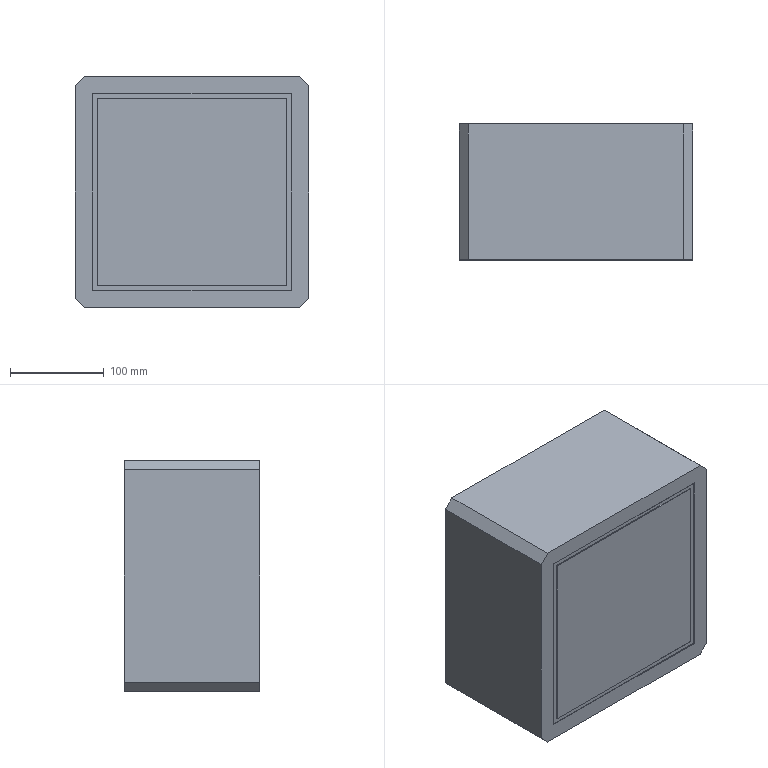Part | SolidWorks | features Chamfer 1, Extrusion 1, ICE 1 | 1 solid | 20 faces | box 250 x 145 x 247 mm | volume 8920630 mm3 | plane 20
STEP:
#1=CARTESIAN_POINT('',(125.,145.,113.5));
#2=VERTEX_POINT('',#1);
#3=CARTESIAN_POINT('',(125.,145.,-113.5));
#4=VERTEX_POINT('',#3);
#5=CARTESIAN_POINT('',(125.,145.,123.5));
#6=DIRECTION('',(0.,0.,-1.));
#7=VECTOR('',#6,1000.);
#8=LINE('',#5,#7);
#9=EDGE_CURVE('',#2,#4,#8,.T.);
#10=ORIENTED_EDGE('',*,*,#9,.F.);
#11=CARTESIAN_POINT('',(125.,0.,113.5));
#12=VERTEX_POINT('',#11);
#13=CARTESIAN_POINT('',(125.,145.,113.5));
#14=DIRECTION('',(0.,-1.,0.));
#15=VECTOR('',#14,1000.);
#16=LINE('',#13,#15);
#17=EDGE_CURVE('',#2,#12,#16,.T.);
#18=ORIENTED_EDGE('',*,*,#17,.T.);
#19=CARTESIAN_POINT('',(125.,0.,-113.5));
#20=VERTEX_POINT('',#19);
#21=CARTESIAN_POINT('',(125.,0.,123.5));
#22=DIRECTION('',(0.,0.,-1.));
#23=VECTOR('',#22,1000.);
#24=LINE('',#21,#23);
#25=EDGE_CURVE('',#12,#20,#24,.T.);
#26=ORIENTED_EDGE('',*,*,#25,.T.);
#27=CARTESIAN_POINT('',(125.,145.,-113.5));
#28=DIRECTION('',(0.,1.,0.));
#29=VECTOR('',#28,1000.);
#30=LINE('',#27,#29);
#31=EDGE_CURVE('',#20,#4,#30,.T.);
#32=ORIENTED_EDGE('',*,*,#31,.T.);
#33=EDGE_LOOP('',(#10,#18,#26,#32));
#34=FACE_OUTER_BOUND('',#33,.T.);
#35=CARTESIAN_POINT('',(125.,145.,123.5));
#36=DIRECTION('',(-1.,0.,0.));
#37=DIRECTION('',(0.,0.,1.));
#38=AXIS2_PLACEMENT_3D('',#35,#36,#37);
#39=PLANE('',#38);
#40=ADVANCED_FACE('',(#34),#39,.F.);
#41=CARTESIAN_POINT('',(115.,145.,-123.5));
#42=VERTEX_POINT('',#41);
#43=CARTESIAN_POINT('',(-115.,145.,-123.5));
#44=VERTEX_POINT('',#43);
#45=CARTESIAN_POINT('',(-125.,145.,-123.5));
#46=DIRECTION('',(-1.,0.,0.));
#47=VECTOR('',#46,1000.);
#48=LINE('',#45,#47);
#49=EDGE_CURVE('',#42,#44,#48,.T.);
#50=ORIENTED_EDGE('',*,*,#49,.F.);
#51=CARTESIAN_POINT('',(115.,0.,-123.5));
#52=VERTEX_POINT('',#51);
#53=CARTESIAN_POINT('',(115.,145.,-123.5));
#54=DIRECTION('',(0.,-1.,0.));
#55=VECTOR('',#54,1000.);
#56=LINE('',#53,#55);
#57=EDGE_CURVE('',#42,#52,#56,.T.);
#58=ORIENTED_EDGE('',*,*,#57,.T.);
#59=CARTESIAN_POINT('',(-115.,0.,-123.5));
#60=VERTEX_POINT('',#59);
#61=CARTESIAN_POINT('',(-125.,0.,-123.5));
#62=DIRECTION('',(-1.,0.,0.));
#63=VECTOR('',#62,1000.);
#64=LINE('',#61,#63);
#65=EDGE_CURVE('',#52,#60,#64,.T.);
#66=ORIENTED_EDGE('',*,*,#65,.T.);
#67=CARTESIAN_POINT('',(-115.,145.,-123.5));
#68=DIRECTION('',(0.,1.,0.));
#69=VECTOR('',#68,1000.);
#70=LINE('',#67,#69);
#71=EDGE_CURVE('',#60,#44,#70,.T.);
#72=ORIENTED_EDGE('',*,*,#71,.T.);
#73=EDGE_LOOP('',(#50,#58,#66,#72));
#74=FACE_OUTER_BOUND('',#73,.T.);
#75=CARTESIAN_POINT('',(-125.,145.,-123.5));
#76=DIRECTION('',(0.,0.,1.));
#77=DIRECTION('',(1.,0.,0.));
#78=AXIS2_PLACEMENT_3D('',#75,#76,#77);
#79=PLANE('',#78);
#80=ADVANCED_FACE('',(#74),#79,.F.);
#81=CARTESIAN_POINT('',(-125.,145.,-113.5));
#82=VERTEX_POINT('',#81);
#83=CARTESIAN_POINT('',(-125.,145.,113.5));
#84=VERTEX_POINT('',#83);
#85=CARTESIAN_POINT('',(-125.,145.,123.5));
#86=DIRECTION('',(0.,0.,1.));
#87=VECTOR('',#86,1000.);
#88=LINE('',#85,#87);
#89=EDGE_CURVE('',#82,#84,#88,.T.);
#90=ORIENTED_EDGE('',*,*,#89,.F.);
#91=CARTESIAN_POINT('',(-125.,0.,-113.5));
#92=VERTEX_POINT('',#91);
#93=CARTESIAN_POINT('',(-125.,145.,-113.5));
#94=DIRECTION('',(0.,-1.,0.));
#95=VECTOR('',#94,1000.);
#96=LINE('',#93,#95);
#97=EDGE_CURVE('',#82,#92,#96,.T.);
#98=ORIENTED_EDGE('',*,*,#97,.T.);
#99=CARTESIAN_POINT('',(-125.,0.,113.5));
#100=VERTEX_POINT('',#99);
#101=CARTESIAN_POINT('',(-125.,0.,123.5));
#102=DIRECTION('',(0.,0.,1.));
#103=VECTOR('',#102,1000.);
#104=LINE('',#101,#103);
#105=EDGE_CURVE('',#92,#100,#104,.T.);
#106=ORIENTED_EDGE('',*,*,#105,.T.);
#107=CARTESIAN_POINT('',(-125.,145.,113.5));
#108=DIRECTION('',(0.,1.,0.));
#109=VECTOR('',#108,1000.);
#110=LINE('',#107,#109);
#111=EDGE_CURVE('',#100,#84,#110,.T.);
#112=ORIENTED_EDGE('',*,*,#111,.T.);
#113=EDGE_LOOP('',(#90,#98,#106,#112));
#114=FACE_OUTER_BOUND('',#113,.T.);
#115=CARTESIAN_POINT('',(-125.,145.,123.5));
#116=DIRECTION('',(1.,0.,0.));
#117=DIRECTION('',(0.,0.,-1.));
#118=AXIS2_PLACEMENT_3D('',#115,#116,#117);
#119=PLANE('',#118);
#120=ADVANCED_FACE('',(#114),#119,.F.);
#121=CARTESIAN_POINT('',(-115.,0.,123.5));
#122=VERTEX_POINT('',#121);
#123=CARTESIAN_POINT('',(115.,0.,123.5));
#124=VERTEX_POINT('',#123);
#125=CARTESIAN_POINT('',(-125.,0.,123.5));
#126=DIRECTION('',(1.,0.,0.));
#127=VECTOR('',#126,1000.);
#128=LINE('',#125,#127);
#129=EDGE_CURVE('',#122,#124,#128,.T.);
#130=ORIENTED_EDGE('',*,*,#129,.T.);
#131=CARTESIAN_POINT('',(115.,145.,123.5));
#132=VERTEX_POINT('',#131);
#133=CARTESIAN_POINT('',(115.,145.,123.5));
#134=DIRECTION('',(0.,1.,0.));
#135=VECTOR('',#134,1000.);
#136=LINE('',#133,#135);
#137=EDGE_CURVE('',#124,#132,#136,.T.);
#138=ORIENTED_EDGE('',*,*,#137,.T.);
#139=CARTESIAN_POINT('',(-115.,145.,123.5));
#140=VERTEX_POINT('',#139);
#141=CARTESIAN_POINT('',(-125.,145.,123.5));
#142=DIRECTION('',(1.,0.,0.));
#143=VECTOR('',#142,1000.);
#144=LINE('',#141,#143);
#145=EDGE_CURVE('',#140,#132,#144,.T.);
#146=ORIENTED_EDGE('',*,*,#145,.F.);
#147=CARTESIAN_POINT('',(-115.,145.,123.5));
#148=DIRECTION('',(0.,-1.,0.));
#149=VECTOR('',#148,1000.);
#150=LINE('',#147,#149);
#151=EDGE_CURVE('',#140,#122,#150,.T.);
#152=ORIENTED_EDGE('',*,*,#151,.T.);
#153=EDGE_LOOP('',(#130,#138,#146,#152));
#154=FACE_OUTER_BOUND('',#153,.T.);
#155=CARTESIAN_POINT('',(-125.,145.,123.5));
#156=DIRECTION('',(0.,0.,-1.));
#157=DIRECTION('',(-1.,0.,0.));
#158=AXIS2_PLACEMENT_3D('',#155,#156,#157);
#159=PLANE('',#158);
#160=ADVANCED_FACE('',(#154),#159,.F.);
#161=ORIENTED_EDGE('',*,*,#145,.T.);
#162=CARTESIAN_POINT('',(125.,145.,113.5));
#163=DIRECTION('',(0.7071,0.,-0.7071));
#164=VECTOR('',#163,1000.);
#165=LINE('',#162,#164);
#166=EDGE_CURVE('',#132,#2,#165,.T.);
#167=ORIENTED_EDGE('',*,*,#166,.T.);
#168=ORIENTED_EDGE('',*,*,#9,.T.);
#169=CARTESIAN_POINT('',(115.,145.,-123.5));
#170=DIRECTION('',(-0.7071,0.,-0.7071));
#171=VECTOR('',#170,1000.);
#172=LINE('',#169,#171);
#173=EDGE_CURVE('',#4,#42,#172,.T.);
#174=ORIENTED_EDGE('',*,*,#173,.T.);
#175=ORIENTED_EDGE('',*,*,#49,.T.);
#176=CARTESIAN_POINT('',(-125.,145.,-113.5));
#177=DIRECTION('',(-0.7071,0.,0.7071));
#178=VECTOR('',#177,1000.);
#179=LINE('',#176,#178);
#180=EDGE_CURVE('',#44,#82,#179,.T.);
#181=ORIENTED_EDGE('',*,*,#180,.T.);
#182=ORIENTED_EDGE('',*,*,#89,.T.);
#183=CARTESIAN_POINT('',(-115.,145.,123.5));
#184=DIRECTION('',(0.7071,0.,0.7071));
#185=VECTOR('',#184,1000.);
#186=LINE('',#183,#185);
#187=EDGE_CURVE('',#84,#140,#186,.T.);
#188=ORIENTED_EDGE('',*,*,#187,.T.);
#189=EDGE_LOOP('',(#161,#167,#168,#174,#175,#181,#182,#188));
#190=FACE_OUTER_BOUND('',#189,.T.);
#191=CARTESIAN_POINT('',(0.,145.,0.));
#192=DIRECTION('',(0.,-1.,0.));
#193=DIRECTION('',(0.,0.,-1.));
#194=AXIS2_PLACEMENT_3D('',#191,#192,#193);
#195=PLANE('',#194);
#196=ADVANCED_FACE('',(#190),#195,.F.);
#197=CARTESIAN_POINT('',(106.,0.,-105.));
#198=VERTEX_POINT('',#197);
#199=CARTESIAN_POINT('',(106.,0.,105.));
#200=VERTEX_POINT('',#199);
#201=CARTESIAN_POINT('',(106.,0.,-105.));
#202=DIRECTION('',(0.,0.,1.));
#203=VECTOR('',#202,1000.);
#204=LINE('',#201,#203);
#205=EDGE_CURVE('',#198,#200,#204,.T.);
#206=ORIENTED_EDGE('',*,*,#205,.F.);
#207=CARTESIAN_POINT('',(-106.,0.,-105.));
#208=VERTEX_POINT('',#207);
#209=CARTESIAN_POINT('',(-106.,0.,-105.));
#210=DIRECTION('',(1.,0.,0.));
#211=VECTOR('',#210,1000.);
#212=LINE('',#209,#211);
#213=EDGE_CURVE('',#208,#198,#212,.T.);
#214=ORIENTED_EDGE('',*,*,#213,.F.);
#215=CARTESIAN_POINT('',(-106.,0.,105.));
#216=VERTEX_POINT('',#215);
#217=CARTESIAN_POINT('',(-106.,0.,-105.));
#218=DIRECTION('',(0.,0.,-1.));
#219=VECTOR('',#218,1000.);
#220=LINE('',#217,#219);
#221=EDGE_CURVE('',#216,#208,#220,.T.);
#222=ORIENTED_EDGE('',*,*,#221,.F.);
#223=CARTESIAN_POINT('',(-106.,0.,105.));
#224=DIRECTION('',(-1.,0.,0.));
#225=VECTOR('',#224,1000.);
#226=LINE('',#223,#225);
#227=EDGE_CURVE('',#200,#216,#226,.T.);
#228=ORIENTED_EDGE('',*,*,#227,.F.);
#229=EDGE_LOOP('',(#206,#214,#222,#228));
#230=FACE_BOUND('',#229,.T.);
#231=ORIENTED_EDGE('',*,*,#25,.F.);
#232=CARTESIAN_POINT('',(119.25,0.,119.25));
#233=DIRECTION('',(-0.7071,0.,0.7071));
#234=VECTOR('',#233,1000.);
#235=LINE('',#232,#234);
#236=EDGE_CURVE('',#12,#124,#235,.T.);
#237=ORIENTED_EDGE('',*,*,#236,.T.);
#238=ORIENTED_EDGE('',*,*,#129,.F.);
#239=CARTESIAN_POINT('',(-119.25,0.,119.25));
#240=DIRECTION('',(-0.7071,0.,-0.7071));
#241=VECTOR('',#240,1000.);
#242=LINE('',#239,#241);
#243=EDGE_CURVE('',#122,#100,#242,.T.);
#244=ORIENTED_EDGE('',*,*,#243,.T.);
#245=ORIENTED_EDGE('',*,*,#105,.F.);
#246=CARTESIAN_POINT('',(-119.25,0.,-119.25));
#247=DIRECTION('',(0.7071,0.,-0.7071));
#248=VECTOR('',#247,1000.);
#249=LINE('',#246,#248);
#250=EDGE_CURVE('',#92,#60,#249,.T.);
#251=ORIENTED_EDGE('',*,*,#250,.T.);
#252=ORIENTED_EDGE('',*,*,#65,.F.);
#253=CARTESIAN_POINT('',(119.25,0.,-119.25));
#254=DIRECTION('',(0.7071,0.,0.7071));
#255=VECTOR('',#254,1000.);
#256=LINE('',#253,#255);
#257=EDGE_CURVE('',#52,#20,#256,.T.);
#258=ORIENTED_EDGE('',*,*,#257,.T.);
#259=EDGE_LOOP('',(#231,#237,#238,#244,#245,#251,#252,#258));
#260=FACE_OUTER_BOUND('',#259,.T.);
#261=CARTESIAN_POINT('',(0.,0.,0.));
#262=DIRECTION('',(0.,-1.,0.));
#263=DIRECTION('',(0.,0.,-1.));
#264=AXIS2_PLACEMENT_3D('',#261,#262,#263);
#265=PLANE('',#264);
#266=ADVANCED_FACE('',(#230,#260),#265,.T.);
#267=ORIENTED_EDGE('',*,*,#166,.F.);
#268=ORIENTED_EDGE('',*,*,#137,.F.);
#269=ORIENTED_EDGE('',*,*,#236,.F.);
#270=ORIENTED_EDGE('',*,*,#17,.F.);
#271=EDGE_LOOP('',(#267,#268,#269,#270));
#272=FACE_OUTER_BOUND('',#271,.T.);
#273=CARTESIAN_POINT('',(125.,145.,113.5));
#274=DIRECTION('',(-0.7071,0.,-0.7071));
#275=DIRECTION('',(0.,-1.,0.));
#276=AXIS2_PLACEMENT_3D('',#273,#274,#275);
#277=PLANE('',#276);
#278=ADVANCED_FACE('',(#272),#277,.F.);
#279=ORIENTED_EDGE('',*,*,#173,.F.);
#280=ORIENTED_EDGE('',*,*,#31,.F.);
#281=ORIENTED_EDGE('',*,*,#257,.F.);
#282=ORIENTED_EDGE('',*,*,#57,.F.);
#283=EDGE_LOOP('',(#279,#280,#281,#282));
#284=FACE_OUTER_BOUND('',#283,.T.);
#285=CARTESIAN_POINT('',(115.,145.,-123.5));
#286=DIRECTION('',(-0.7071,0.,0.7071));
#287=DIRECTION('',(0.,-1.,0.));
#288=AXIS2_PLACEMENT_3D('',#285,#286,#287);
#289=PLANE('',#288);
#290=ADVANCED_FACE('',(#284),#289,.F.);
#291=ORIENTED_EDGE('',*,*,#180,.F.);
#292=ORIENTED_EDGE('',*,*,#71,.F.);
#293=ORIENTED_EDGE('',*,*,#250,.F.);
#294=ORIENTED_EDGE('',*,*,#97,.F.);
#295=EDGE_LOOP('',(#291,#292,#293,#294));
#296=FACE_OUTER_BOUND('',#295,.T.);
#297=CARTESIAN_POINT('',(-125.,145.,-113.5));
#298=DIRECTION('',(0.7071,0.,0.7071));
#299=DIRECTION('',(0.,-1.,0.));
#300=AXIS2_PLACEMENT_3D('',#297,#298,#299);
#301=PLANE('',#300);
#302=ADVANCED_FACE('',(#296),#301,.F.);
#303=ORIENTED_EDGE('',*,*,#187,.F.);
#304=ORIENTED_EDGE('',*,*,#111,.F.);
#305=ORIENTED_EDGE('',*,*,#243,.F.);
#306=ORIENTED_EDGE('',*,*,#151,.F.);
#307=EDGE_LOOP('',(#303,#304,#305,#306));
#308=FACE_OUTER_BOUND('',#307,.T.);
#309=CARTESIAN_POINT('',(-115.,145.,123.5));
#310=DIRECTION('',(0.7071,0.,-0.7071));
#311=DIRECTION('',(0.,-1.,0.));
#312=AXIS2_PLACEMENT_3D('',#309,#310,#311);
#313=PLANE('',#312);
#314=ADVANCED_FACE('',(#308),#313,.F.);
#315=ORIENTED_EDGE('',*,*,#205,.T.);
#316=CARTESIAN_POINT('',(106.,1.,105.));
#317=VERTEX_POINT('',#316);
#318=CARTESIAN_POINT('',(106.,1.,105.));
#319=DIRECTION('',(0.,-1.,0.));
#320=VECTOR('',#319,1000.);
#321=LINE('',#318,#320);
#322=EDGE_CURVE('',#317,#200,#321,.T.);
#323=ORIENTED_EDGE('',*,*,#322,.F.);
#324=CARTESIAN_POINT('',(106.,1.,-105.));
#325=VERTEX_POINT('',#324);
#326=CARTESIAN_POINT('',(106.,1.,-105.));
#327=DIRECTION('',(0.,0.,1.));
#328=VECTOR('',#327,1000.);
#329=LINE('',#326,#328);
#330=EDGE_CURVE('',#325,#317,#329,.T.);
#331=ORIENTED_EDGE('',*,*,#330,.F.);
#332=CARTESIAN_POINT('',(106.,1.,-105.));
#333=DIRECTION('',(0.,-1.,0.));
#334=VECTOR('',#333,1000.);
#335=LINE('',#332,#334);
#336=EDGE_CURVE('',#325,#198,#335,.T.);
#337=ORIENTED_EDGE('',*,*,#336,.T.);
#338=EDGE_LOOP('',(#315,#323,#331,#337));
#339=FACE_OUTER_BOUND('',#338,.T.);
#340=CARTESIAN_POINT('',(106.,1.,-105.));
#341=DIRECTION('',(1.,0.,0.));
#342=DIRECTION('',(0.,0.,-1.));
#343=AXIS2_PLACEMENT_3D('',#340,#341,#342);
#344=PLANE('',#343);
#345=ADVANCED_FACE('',(#339),#344,.F.);
#346=ORIENTED_EDGE('',*,*,#213,.T.);
#347=ORIENTED_EDGE('',*,*,#336,.F.);
#348=CARTESIAN_POINT('',(-106.,1.,-105.));
#349=VERTEX_POINT('',#348);
#350=CARTESIAN_POINT('',(-106.,1.,-105.));
#351=DIRECTION('',(1.,0.,0.));
#352=VECTOR('',#351,1000.);
#353=LINE('',#350,#352);
#354=EDGE_CURVE('',#349,#325,#353,.T.);
#355=ORIENTED_EDGE('',*,*,#354,.F.);
#356=CARTESIAN_POINT('',(-106.,1.,-105.));
#357=DIRECTION('',(0.,-1.,0.));
#358=VECTOR('',#357,1000.);
#359=LINE('',#356,#358);
#360=EDGE_CURVE('',#349,#208,#359,.T.);
#361=ORIENTED_EDGE('',*,*,#360,.T.);
#362=EDGE_LOOP('',(#346,#347,#355,#361));
#363=FACE_OUTER_BOUND('',#362,.T.);
#364=CARTESIAN_POINT('',(-106.,1.,-105.));
#365=DIRECTION('',(0.,0.,-1.));
#366=DIRECTION('',(-1.,0.,0.));
#367=AXIS2_PLACEMENT_3D('',#364,#365,#366);
#368=PLANE('',#367);
#369=ADVANCED_FACE('',(#363),#368,.F.);
#370=ORIENTED_EDGE('',*,*,#221,.T.);
#371=ORIENTED_EDGE('',*,*,#360,.F.);
#372=CARTESIAN_POINT('',(-106.,1.,105.));
#373=VERTEX_POINT('',#372);
#374=CARTESIAN_POINT('',(-106.,1.,-105.));
#375=DIRECTION('',(0.,0.,-1.));
#376=VECTOR('',#375,1000.);
#377=LINE('',#374,#376);
#378=EDGE_CURVE('',#373,#349,#377,.T.);
#379=ORIENTED_EDGE('',*,*,#378,.F.);
#380=CARTESIAN_POINT('',(-106.,1.,105.));
#381=DIRECTION('',(0.,-1.,0.));
#382=VECTOR('',#381,1000.);
#383=LINE('',#380,#382);
#384=EDGE_CURVE('',#373,#216,#383,.T.);
#385=ORIENTED_EDGE('',*,*,#384,.T.);
#386=EDGE_LOOP('',(#370,#371,#379,#385));
#387=FACE_OUTER_BOUND('',#386,.T.);
#388=CARTESIAN_POINT('',(-106.,1.,-105.));
#389=DIRECTION('',(-1.,0.,0.));
#390=DIRECTION('',(0.,0.,1.));
#391=AXIS2_PLACEMENT_3D('',#388,#389,#390);
#392=PLANE('',#391);
#393=ADVANCED_FACE('',(#387),#392,.F.);
#394=ORIENTED_EDGE('',*,*,#227,.T.);
#395=ORIENTED_EDGE('',*,*,#384,.F.);
#396=CARTESIAN_POINT('',(-106.,1.,105.));
#397=DIRECTION('',(-1.,0.,0.));
#398=VECTOR('',#397,1000.);
#399=LINE('',#396,#398);
#400=EDGE_CURVE('',#317,#373,#399,.T.);
#401=ORIENTED_EDGE('',*,*,#400,.F.);
#402=ORIENTED_EDGE('',*,*,#322,.T.);
#403=EDGE_LOOP('',(#394,#395,#401,#402));
#404=FACE_OUTER_BOUND('',#403,.T.);
#405=CARTESIAN_POINT('',(-106.,1.,105.));
#406=DIRECTION('',(0.,0.,1.));
#407=DIRECTION('',(1.,0.,0.));
#408=AXIS2_PLACEMENT_3D('',#405,#406,#407);
#409=PLANE('',#408);
#410=ADVANCED_FACE('',(#404),#409,.F.);
#411=CARTESIAN_POINT('',(-101.,1.,-100.));
#412=VERTEX_POINT('',#411);
#413=CARTESIAN_POINT('',(101.,1.,-100.));
#414=VERTEX_POINT('',#413);
#415=CARTESIAN_POINT('',(-101.,1.,-100.));
#416=DIRECTION('',(1.,0.,0.));
#417=VECTOR('',#416,1000.);
#418=LINE('',#415,#417);
#419=EDGE_CURVE('',#412,#414,#418,.T.);
#420=ORIENTED_EDGE('',*,*,#419,.F.);
#421=CARTESIAN_POINT('',(-101.,1.,100.));
#422=VERTEX_POINT('',#421);
#423=CARTESIAN_POINT('',(-101.,1.,-100.));
#424=DIRECTION('',(0.,0.,-1.));
#425=VECTOR('',#424,1000.);
#426=LINE('',#423,#425);
#427=EDGE_CURVE('',#422,#412,#426,.T.);
#428=ORIENTED_EDGE('',*,*,#427,.F.);
#429=CARTESIAN_POINT('',(101.,1.,100.));
#430=VERTEX_POINT('',#429);
#431=CARTESIAN_POINT('',(-101.,1.,100.));
#432=DIRECTION('',(-1.,0.,0.));
#433=VECTOR('',#432,1000.);
#434=LINE('',#431,#433);
#435=EDGE_CURVE('',#430,#422,#434,.T.);
#436=ORIENTED_EDGE('',*,*,#435,.F.);
#437=CARTESIAN_POINT('',(101.,1.,-100.));
#438=DIRECTION('',(0.,0.,1.));
#439=VECTOR('',#438,1000.);
#440=LINE('',#437,#439);
#441=EDGE_CURVE('',#414,#430,#440,.T.);
#442=ORIENTED_EDGE('',*,*,#441,.F.);
#443=EDGE_LOOP('',(#420,#428,#436,#442));
#444=FACE_BOUND('',#443,.T.);
#445=ORIENTED_EDGE('',*,*,#330,.T.);
#446=ORIENTED_EDGE('',*,*,#400,.T.);
#447=ORIENTED_EDGE('',*,*,#378,.T.);
#448=ORIENTED_EDGE('',*,*,#354,.T.);
#449=EDGE_LOOP('',(#445,#446,#447,#448));
#450=FACE_OUTER_BOUND('',#449,.T.);
#451=CARTESIAN_POINT('',(0.,1.,0.));
#452=DIRECTION('',(0.,1.,0.));
#453=DIRECTION('',(0.,0.,1.));
#454=AXIS2_PLACEMENT_3D('',#451,#452,#453);
#455=PLANE('',#454);
#456=ADVANCED_FACE('',(#444,#450),#455,.F.);
#457=CARTESIAN_POINT('',(-101.,0.,-100.));
#458=VERTEX_POINT('',#457);
#459=CARTESIAN_POINT('',(101.,0.,-100.));
#460=VERTEX_POINT('',#459);
#461=CARTESIAN_POINT('',(-101.,0.,-100.));
#462=DIRECTION('',(1.,0.,0.));
#463=VECTOR('',#462,1000.);
#464=LINE('',#461,#463);
#465=EDGE_CURVE('',#458,#460,#464,.T.);
#466=ORIENTED_EDGE('',*,*,#465,.F.);
#467=CARTESIAN_POINT('',(-101.,1.,-100.));
#468=DIRECTION('',(0.,-1.,0.));
#469=VECTOR('',#468,1000.);
#470=LINE('',#467,#469);
#471=EDGE_CURVE('',#412,#458,#470,.T.);
#472=ORIENTED_EDGE('',*,*,#471,.F.);
#473=ORIENTED_EDGE('',*,*,#419,.T.);
#474=CARTESIAN_POINT('',(101.,1.,-100.));
#475=DIRECTION('',(0.,-1.,0.));
#476=VECTOR('',#475,1000.);
#477=LINE('',#474,#476);
#478=EDGE_CURVE('',#414,#460,#477,.T.);
#479=ORIENTED_EDGE('',*,*,#478,.T.);
#480=EDGE_LOOP('',(#466,#472,#473,#479));
#481=FACE_OUTER_BOUND('',#480,.T.);
#482=CARTESIAN_POINT('',(-101.,1.,-100.));
#483=DIRECTION('',(0.,0.,-1.));
#484=DIRECTION('',(-1.,0.,0.));
#485=AXIS2_PLACEMENT_3D('',#482,#483,#484);
#486=PLANE('',#485);
#487=ADVANCED_FACE('',(#481),#486,.T.);
#488=CARTESIAN_POINT('',(-101.,0.,100.));
#489=VERTEX_POINT('',#488);
#490=CARTESIAN_POINT('',(-101.,0.,-100.));
#491=DIRECTION('',(0.,0.,-1.));
#492=VECTOR('',#491,1000.);
#493=LINE('',#490,#492);
#494=EDGE_CURVE('',#489,#458,#493,.T.);
#495=ORIENTED_EDGE('',*,*,#494,.F.);
#496=CARTESIAN_POINT('',(-101.,1.,100.));
#497=DIRECTION('',(0.,-1.,0.));
#498=VECTOR('',#497,1000.);
#499=LINE('',#496,#498);
#500=EDGE_CURVE('',#422,#489,#499,.T.);
#501=ORIENTED_EDGE('',*,*,#500,.F.);
#502=ORIENTED_EDGE('',*,*,#427,.T.);
#503=ORIENTED_EDGE('',*,*,#471,.T.);
#504=EDGE_LOOP('',(#495,#501,#502,#503));
#505=FACE_OUTER_BOUND('',#504,.T.);
#506=CARTESIAN_POINT('',(-101.,1.,-100.));
#507=DIRECTION('',(-1.,0.,0.));
#508=DIRECTION('',(0.,0.,1.));
#509=AXIS2_PLACEMENT_3D('',#506,#507,#508);
#510=PLANE('',#509);
#511=ADVANCED_FACE('',(#505),#510,.T.);
#512=CARTESIAN_POINT('',(101.,0.,100.));
#513=VERTEX_POINT('',#512);
#514=CARTESIAN_POINT('',(-101.,0.,100.));
#515=DIRECTION('',(-1.,0.,0.));
#516=VECTOR('',#515,1000.);
#517=LINE('',#514,#516);
#518=EDGE_CURVE('',#513,#489,#517,.T.);
#519=ORIENTED_EDGE('',*,*,#518,.F.);
#520=CARTESIAN_POINT('',(101.,1.,100.));
#521=DIRECTION('',(0.,-1.,0.));
#522=VECTOR('',#521,1000.);
#523=LINE('',#520,#522);
#524=EDGE_CURVE('',#430,#513,#523,.T.);
#525=ORIENTED_EDGE('',*,*,#524,.F.);
#526=ORIENTED_EDGE('',*,*,#435,.T.);
#527=ORIENTED_EDGE('',*,*,#500,.T.);
#528=EDGE_LOOP('',(#519,#525,#526,#527));
#529=FACE_OUTER_BOUND('',#528,.T.);
#530=CARTESIAN_POINT('',(-101.,1.,100.));
#531=DIRECTION('',(0.,0.,1.));
#532=DIRECTION('',(1.,0.,0.));
#533=AXIS2_PLACEMENT_3D('',#530,#531,#532);
#534=PLANE('',#533);
#535=ADVANCED_FACE('',(#529),#534,.T.);
#536=CARTESIAN_POINT('',(101.,0.,-100.));
#537=DIRECTION('',(0.,0.,1.));
#538=VECTOR('',#537,1000.);
#539=LINE('',#536,#538);
#540=EDGE_CURVE('',#460,#513,#539,.T.);
#541=ORIENTED_EDGE('',*,*,#540,.F.);
#542=ORIENTED_EDGE('',*,*,#478,.F.);
#543=ORIENTED_EDGE('',*,*,#441,.T.);
#544=ORIENTED_EDGE('',*,*,#524,.T.);
#545=EDGE_LOOP('',(#541,#542,#543,#544));
#546=FACE_OUTER_BOUND('',#545,.T.);
#547=CARTESIAN_POINT('',(101.,1.,-100.));
#548=DIRECTION('',(1.,0.,0.));
#549=DIRECTION('',(0.,0.,-1.));
#550=AXIS2_PLACEMENT_3D('',#547,#548,#549);
#551=PLANE('',#550);
#552=ADVANCED_FACE('',(#546),#551,.T.);
#553=ORIENTED_EDGE('',*,*,#494,.T.);
#554=ORIENTED_EDGE('',*,*,#465,.T.);
#555=ORIENTED_EDGE('',*,*,#540,.T.);
#556=ORIENTED_EDGE('',*,*,#518,.T.);
#557=EDGE_LOOP('',(#553,#554,#555,#556));
#558=FACE_OUTER_BOUND('',#557,.T.);
#559=CARTESIAN_POINT('',(0.,0.,0.));
#560=DIRECTION('',(0.,-1.,0.));
#561=DIRECTION('',(0.,0.,-1.));
#562=AXIS2_PLACEMENT_3D('',#559,#560,#561);
#563=PLANE('',#562);
#564=ADVANCED_FACE('',(#558),#563,.T.);
#565=CLOSED_SHELL('',(#40,#80,#120,#160,#196,#266,#278,#290,#302,#314,#345,#369,#393,#410,#456,#487,#511,#535,#552,#564));
#566=MANIFOLD_SOLID_BREP('',#565);
#567=CARTESIAN_POINT('',(0.,0.,0.));
#568=DIRECTION('',(0.,0.,1.));
#569=DIRECTION('',(1.,0.,0.));
#570=AXIS2_PLACEMENT_3D('',#567,#568,#569);
#571=(LENGTH_UNIT()NAMED_UNIT(*)SI_UNIT(.MILLI.,.METRE.));
#572=UNCERTAINTY_MEASURE_WITH_UNIT(LENGTH_MEASURE(0.00001),#571,'','');
#573=(NAMED_UNIT(*)PLANE_ANGLE_UNIT()SI_UNIT($,.RADIAN.));
#574=(NAMED_UNIT(*)SI_UNIT($,.STERADIAN.)SOLID_ANGLE_UNIT());
#575=(GEOMETRIC_REPRESENTATION_CONTEXT(3)GLOBAL_UNCERTAINTY_ASSIGNED_CONTEXT((#572))GLOBAL_UNIT_ASSIGNED_CONTEXT((#571,#573,#574))REPRESENTATION_CONTEXT('',''));
#576=ADVANCED_BREP_SHAPE_REPRESENTATION('',(#566,#570),#575);